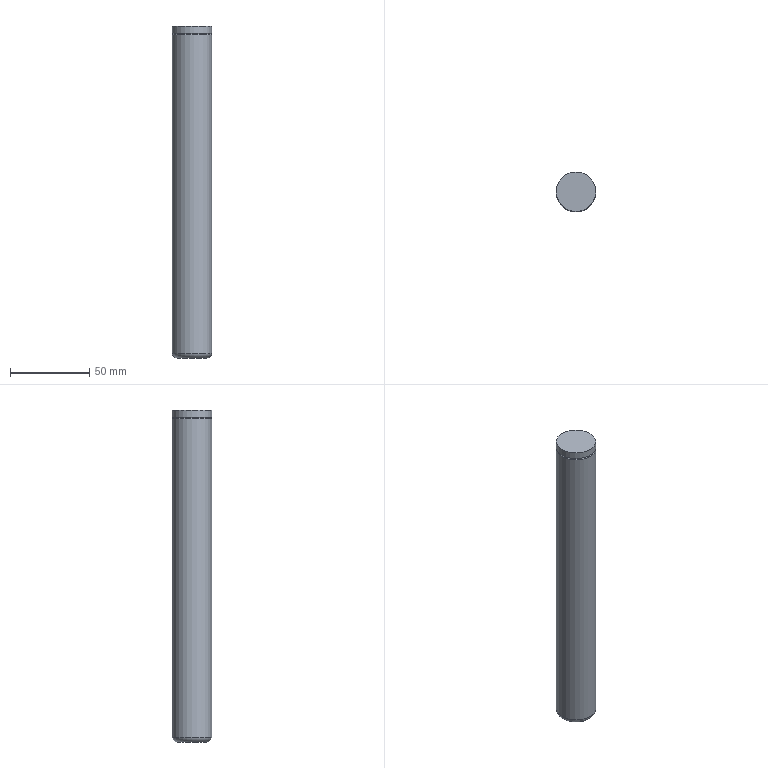Part | STEP file | 1 solid | 6 faces | box 25 x 25 x 210 mm | volume 102898 mm3 | plane 2 | cylinder 2 | torus 2 | commonest cylinder face diameters 25 x2
STEP:
#1=CARTESIAN_POINT('',(0.,0.,0.));
#2=DIRECTION('',(0.,0.,1.));
#3=DIRECTION('',(1.,0.,0.));
#4=AXIS2_PLACEMENT_3D('',#1,#2,#3);
#5=CARTESIAN_POINT('',(1301.872,580.48,-116.381));
#6=VERTEX_POINT('',#5);
#7=CARTESIAN_POINT('',(1311.247,580.48,-116.381));
#8=DIRECTION('',(0.,0.,-1.));
#9=DIRECTION('',(-1.,0.,0.));
#10=AXIS2_PLACEMENT_3D('',#7,#8,#9);
#11=CIRCLE('',#10,9.375);
#12=CARTESIAN_POINT('',(1311.247,580.48,-116.381));
#13=DIRECTION('',(0.,0.,-1.));
#14=DIRECTION('',(-1.,0.,0.));
#15=AXIS2_PLACEMENT_3D('',#12,#13,#14);
#16=PLANE('',#15);
#17=CARTESIAN_POINT('',(0.,0.));
#18=DIRECTION('',(1.,0.));
#19=AXIS2_PLACEMENT_2D('',#17,#18);
#20=CIRCLE('',#19,9.375);
#21=(GEOMETRIC_REPRESENTATION_CONTEXT(2)PARAMETRIC_REPRESENTATION_CONTEXT()REPRESENTATION_CONTEXT('',''));
#22=DEFINITIONAL_REPRESENTATION('',(#20),#21);
#23=PCURVE('',#16,#22);
#24=CARTESIAN_POINT('',(1311.247,580.48,-113.256));
#25=DIRECTION('',(0.,0.,-1.));
#26=DIRECTION('',(-1.,0.,0.));
#27=AXIS2_PLACEMENT_3D('',#24,#25,#26);
#28=TOROIDAL_SURFACE('',#27,9.375,3.125);
#29=CARTESIAN_POINT('',(0.,7.854));
#30=DIRECTION('',(1.,0.));
#31=VECTOR('',#30,1.);
#32=LINE('',#29,#31);
#33=(GEOMETRIC_REPRESENTATION_CONTEXT(2)PARAMETRIC_REPRESENTATION_CONTEXT()REPRESENTATION_CONTEXT('',''));
#34=DEFINITIONAL_REPRESENTATION('',(#32),#33);
#35=PCURVE('',#28,#34);
#36=SURFACE_CURVE('',#11,(#23,#35),.PCURVE_S1.);
#37=EDGE_CURVE('',#6,#6,#36,.T.);
#38=ORIENTED_EDGE('',*,*,#37,.T.);
#39=EDGE_LOOP('',(#38));
#40=FACE_BOUND('',#39,.T.);
#41=ADVANCED_FACE('',(#40),#16,.T.);
#42=CARTESIAN_POINT('',(1323.747,580.48,93.619));
#43=VERTEX_POINT('',#42);
#44=CARTESIAN_POINT('',(1311.247,580.48,93.619));
#45=DIRECTION('',(0.,0.,1.));
#46=DIRECTION('',(1.,0.,0.));
#47=AXIS2_PLACEMENT_3D('',#44,#45,#46);
#48=CIRCLE('',#47,12.5);
#49=CARTESIAN_POINT('',(1311.247,580.48,93.619));
#50=DIRECTION('',(0.,0.,1.));
#51=DIRECTION('',(1.,0.,0.));
#52=AXIS2_PLACEMENT_3D('',#49,#50,#51);
#53=PLANE('',#52);
#54=CARTESIAN_POINT('',(0.,0.));
#55=DIRECTION('',(1.,0.));
#56=AXIS2_PLACEMENT_2D('',#54,#55);
#57=CIRCLE('',#56,12.5);
#58=(GEOMETRIC_REPRESENTATION_CONTEXT(2)PARAMETRIC_REPRESENTATION_CONTEXT()REPRESENTATION_CONTEXT('',''));
#59=DEFINITIONAL_REPRESENTATION('',(#57),#58);
#60=PCURVE('',#53,#59);
#61=CARTESIAN_POINT('',(1311.247,580.48,-116.381));
#62=DIRECTION('',(0.,0.,1.));
#63=DIRECTION('',(1.,0.,0.));
#64=AXIS2_PLACEMENT_3D('',#61,#62,#63);
#65=CYLINDRICAL_SURFACE('',#64,12.5);
#66=CARTESIAN_POINT('',(0.,210.));
#67=DIRECTION('',(1.,0.));
#68=VECTOR('',#67,1.);
#69=LINE('',#66,#68);
#70=(GEOMETRIC_REPRESENTATION_CONTEXT(2)PARAMETRIC_REPRESENTATION_CONTEXT()REPRESENTATION_CONTEXT('',''));
#71=DEFINITIONAL_REPRESENTATION('',(#69),#70);
#72=PCURVE('',#65,#71);
#73=SURFACE_CURVE('',#48,(#60,#72),.PCURVE_S1.);
#74=EDGE_CURVE('',#43,#43,#73,.T.);
#75=ORIENTED_EDGE('',*,*,#74,.T.);
#76=EDGE_LOOP('',(#75));
#77=FACE_BOUND('',#76,.T.);
#78=ADVANCED_FACE('',(#77),#53,.T.);
#79=CARTESIAN_POINT('',(1323.747,580.48,89.119));
#80=VERTEX_POINT('',#79);
#81=CARTESIAN_POINT('',(1311.247,580.48,89.119));
#82=DIRECTION('',(0.,0.,1.));
#83=DIRECTION('',(1.,0.,0.));
#84=AXIS2_PLACEMENT_3D('',#81,#82,#83);
#85=CIRCLE('',#84,12.5);
#86=CARTESIAN_POINT('',(0.,205.5));
#87=DIRECTION('',(1.,0.));
#88=VECTOR('',#87,1.);
#89=LINE('',#86,#88);
#90=(GEOMETRIC_REPRESENTATION_CONTEXT(2)PARAMETRIC_REPRESENTATION_CONTEXT()REPRESENTATION_CONTEXT('',''));
#91=DEFINITIONAL_REPRESENTATION('',(#89),#90);
#92=PCURVE('',#65,#91);
#93=CARTESIAN_POINT('',(1311.247,580.48,88.619));
#94=DIRECTION('',(0.,0.,1.));
#95=DIRECTION('',(1.,0.,0.));
#96=AXIS2_PLACEMENT_3D('',#93,#94,#95);
#97=TOROIDAL_SURFACE('',#96,12.5,0.5);
#98=CARTESIAN_POINT('',(0.,1.571));
#99=DIRECTION('',(1.,0.));
#100=VECTOR('',#99,1.);
#101=LINE('',#98,#100);
#102=(GEOMETRIC_REPRESENTATION_CONTEXT(2)PARAMETRIC_REPRESENTATION_CONTEXT()REPRESENTATION_CONTEXT('',''));
#103=DEFINITIONAL_REPRESENTATION('',(#101),#102);
#104=PCURVE('',#97,#103);
#105=SURFACE_CURVE('',#85,(#92,#104),.PCURVE_S1.);
#106=EDGE_CURVE('',#80,#80,#105,.T.);
#107=ORIENTED_EDGE('',*,*,#106,.T.);
#108=CARTESIAN_POINT('',(1323.747,580.48,89.119));
#109=CARTESIAN_POINT('',(1323.747,580.48,93.619));
#110=B_SPLINE_CURVE_WITH_KNOTS('',1,(#108,#109),.UNSPECIFIED.,.F.,.F.,(2,2),(205.5,210.),.PIECEWISE_BEZIER_KNOTS.);
#111=CARTESIAN_POINT('',(6.283,0.));
#112=DIRECTION('',(0.,1.));
#113=VECTOR('',#112,1.);
#114=LINE('',#111,#113);
#115=(GEOMETRIC_REPRESENTATION_CONTEXT(2)PARAMETRIC_REPRESENTATION_CONTEXT()REPRESENTATION_CONTEXT('',''));
#116=DEFINITIONAL_REPRESENTATION('',(#114),#115);
#117=PCURVE('',#65,#116);
#118=CARTESIAN_POINT('',(0.,0.));
#119=DIRECTION('',(0.,1.));
#120=VECTOR('',#119,1.);
#121=LINE('',#118,#120);
#122=(GEOMETRIC_REPRESENTATION_CONTEXT(2)PARAMETRIC_REPRESENTATION_CONTEXT()REPRESENTATION_CONTEXT('',''));
#123=DEFINITIONAL_REPRESENTATION('',(#121),#122);
#124=PCURVE('',#65,#123);
#125=SEAM_CURVE('',#110,(#117,#124),.PCURVE_S1.);
#126=EDGE_CURVE('',#80,#43,#125,.T.);
#127=ORIENTED_EDGE('',*,*,#126,.T.);
#128=ORIENTED_EDGE('',*,*,#74,.F.);
#129=ORIENTED_EDGE('',*,*,#126,.F.);
#130=EDGE_LOOP('',(#107,#127,#128,#129));
#131=FACE_BOUND('',#130,.T.);
#132=ADVANCED_FACE('',(#131),#65,.T.);
#133=CARTESIAN_POINT('',(1323.747,580.48,88.119));
#134=VERTEX_POINT('',#133);
#135=CARTESIAN_POINT('',(1311.247,580.48,88.119));
#136=DIRECTION('',(0.,0.,1.));
#137=DIRECTION('',(1.,0.,0.));
#138=AXIS2_PLACEMENT_3D('',#135,#136,#137);
#139=CIRCLE('',#138,12.5);
#140=CARTESIAN_POINT('',(0.,4.712));
#141=DIRECTION('',(1.,0.));
#142=VECTOR('',#141,1.);
#143=LINE('',#140,#142);
#144=(GEOMETRIC_REPRESENTATION_CONTEXT(2)PARAMETRIC_REPRESENTATION_CONTEXT()REPRESENTATION_CONTEXT('',''));
#145=DEFINITIONAL_REPRESENTATION('',(#143),#144);
#146=PCURVE('',#97,#145);
#147=CARTESIAN_POINT('',(1311.247,580.48,-116.381));
#148=DIRECTION('',(0.,0.,1.));
#149=DIRECTION('',(1.,0.,0.));
#150=AXIS2_PLACEMENT_3D('',#147,#148,#149);
#151=CYLINDRICAL_SURFACE('',#150,12.5);
#152=CARTESIAN_POINT('',(0.,204.5));
#153=DIRECTION('',(1.,0.));
#154=VECTOR('',#153,1.);
#155=LINE('',#152,#154);
#156=(GEOMETRIC_REPRESENTATION_CONTEXT(2)PARAMETRIC_REPRESENTATION_CONTEXT()REPRESENTATION_CONTEXT('',''));
#157=DEFINITIONAL_REPRESENTATION('',(#155),#156);
#158=PCURVE('',#151,#157);
#159=SURFACE_CURVE('',#139,(#146,#158),.PCURVE_S1.);
#160=EDGE_CURVE('',#134,#134,#159,.T.);
#161=ORIENTED_EDGE('',*,*,#160,.F.);
#162=CARTESIAN_POINT('',(1323.747,580.48,89.119));
#163=CARTESIAN_POINT('',(1323.523,580.48,89.119));
#164=CARTESIAN_POINT('',(1323.299,580.48,89.002));
#165=CARTESIAN_POINT('',(1323.147,580.48,88.767));
#166=CARTESIAN_POINT('',(1323.147,580.48,88.471));
#167=CARTESIAN_POINT('',(1323.299,580.48,88.237));
#168=CARTESIAN_POINT('',(1323.523,580.48,88.119));
#169=CARTESIAN_POINT('',(1323.747,580.48,88.119));
#170=B_SPLINE_CURVE_WITH_KNOTS('',7,(#162,#163,#164,#165,#166,#167,#168,#169),.UNSPECIFIED.,.F.,.F.,(8,8),(1.571,4.712),.PIECEWISE_BEZIER_KNOTS.);
#171=CARTESIAN_POINT('',(0.,0.));
#172=DIRECTION('',(0.,1.));
#173=VECTOR('',#172,1.);
#174=LINE('',#171,#173);
#175=(GEOMETRIC_REPRESENTATION_CONTEXT(2)PARAMETRIC_REPRESENTATION_CONTEXT()REPRESENTATION_CONTEXT('',''));
#176=DEFINITIONAL_REPRESENTATION('',(#174),#175);
#177=PCURVE('',#97,#176);
#178=CARTESIAN_POINT('',(6.283,0.));
#179=DIRECTION('',(0.,1.));
#180=VECTOR('',#179,1.);
#181=LINE('',#178,#180);
#182=(GEOMETRIC_REPRESENTATION_CONTEXT(2)PARAMETRIC_REPRESENTATION_CONTEXT()REPRESENTATION_CONTEXT('',''));
#183=DEFINITIONAL_REPRESENTATION('',(#181),#182);
#184=PCURVE('',#97,#183);
#185=SEAM_CURVE('',#170,(#177,#184),.PCURVE_S1.);
#186=EDGE_CURVE('',#80,#134,#185,.T.);
#187=ORIENTED_EDGE('',*,*,#186,.F.);
#188=ORIENTED_EDGE('',*,*,#106,.T.);
#189=ORIENTED_EDGE('',*,*,#186,.T.);
#190=EDGE_LOOP('',(#161,#187,#188,#189));
#191=FACE_BOUND('',#190,.F.);
#192=ADVANCED_FACE('',(#191),#97,.F.);
#193=CARTESIAN_POINT('',(1298.747,580.48,-113.256));
#194=VERTEX_POINT('',#193);
#195=CARTESIAN_POINT('',(1323.747,580.48,-113.256));
#196=VERTEX_POINT('',#195);
#197=CARTESIAN_POINT('',(1311.247,580.48,-113.256));
#198=DIRECTION('',(0.,0.,1.));
#199=DIRECTION('',(-1.,0.,0.));
#200=AXIS2_PLACEMENT_3D('',#197,#198,#199);
#201=CIRCLE('',#200,12.5);
#202=CARTESIAN_POINT('',(3.142,3.125));
#203=DIRECTION('',(1.,0.));
#204=VECTOR('',#203,1.);
#205=LINE('',#202,#204);
#206=(GEOMETRIC_REPRESENTATION_CONTEXT(2)PARAMETRIC_REPRESENTATION_CONTEXT()REPRESENTATION_CONTEXT('',''));
#207=DEFINITIONAL_REPRESENTATION('',(#205),#206);
#208=PCURVE('',#151,#207);
#209=CARTESIAN_POINT('',(6.283,6.283));
#210=DIRECTION('',(-1.,0.));
#211=VECTOR('',#210,1.);
#212=LINE('',#209,#211);
#213=(GEOMETRIC_REPRESENTATION_CONTEXT(2)PARAMETRIC_REPRESENTATION_CONTEXT()REPRESENTATION_CONTEXT('',''));
#214=DEFINITIONAL_REPRESENTATION('',(#212),#213);
#215=PCURVE('',#28,#214);
#216=SURFACE_CURVE('',#201,(#208,#215),.PCURVE_S1.);
#217=EDGE_CURVE('',#194,#196,#216,.T.);
#218=ORIENTED_EDGE('',*,*,#217,.T.);
#219=CARTESIAN_POINT('',(1323.747,580.48,-113.256));
#220=CARTESIAN_POINT('',(1323.747,580.48,88.119));
#221=B_SPLINE_CURVE_WITH_KNOTS('',1,(#219,#220),.UNSPECIFIED.,.F.,.F.,(2,2),(3.125,204.5),.PIECEWISE_BEZIER_KNOTS.);
#222=CARTESIAN_POINT('',(6.283,0.));
#223=DIRECTION('',(0.,1.));
#224=VECTOR('',#223,1.);
#225=LINE('',#222,#224);
#226=(GEOMETRIC_REPRESENTATION_CONTEXT(2)PARAMETRIC_REPRESENTATION_CONTEXT()REPRESENTATION_CONTEXT('',''));
#227=DEFINITIONAL_REPRESENTATION('',(#225),#226);
#228=PCURVE('',#151,#227);
#229=CARTESIAN_POINT('',(0.,0.));
#230=DIRECTION('',(0.,1.));
#231=VECTOR('',#230,1.);
#232=LINE('',#229,#231);
#233=(GEOMETRIC_REPRESENTATION_CONTEXT(2)PARAMETRIC_REPRESENTATION_CONTEXT()REPRESENTATION_CONTEXT('',''));
#234=DEFINITIONAL_REPRESENTATION('',(#232),#233);
#235=PCURVE('',#151,#234);
#236=SEAM_CURVE('',#221,(#228,#235),.PCURVE_S1.);
#237=EDGE_CURVE('',#196,#134,#236,.T.);
#238=ORIENTED_EDGE('',*,*,#237,.T.);
#239=ORIENTED_EDGE('',*,*,#160,.F.);
#240=ORIENTED_EDGE('',*,*,#237,.F.);
#241=CARTESIAN_POINT('',(1311.247,580.48,-113.256));
#242=DIRECTION('',(0.,0.,1.));
#243=DIRECTION('',(-1.,0.,0.));
#244=AXIS2_PLACEMENT_3D('',#241,#242,#243);
#245=CIRCLE('',#244,12.5);
#246=CARTESIAN_POINT('',(-3.142,3.125));
#247=DIRECTION('',(1.,0.));
#248=VECTOR('',#247,1.);
#249=LINE('',#246,#248);
#250=(GEOMETRIC_REPRESENTATION_CONTEXT(2)PARAMETRIC_REPRESENTATION_CONTEXT()REPRESENTATION_CONTEXT('',''));
#251=DEFINITIONAL_REPRESENTATION('',(#249),#250);
#252=PCURVE('',#151,#251);
#253=CARTESIAN_POINT('',(6.283,6.283));
#254=DIRECTION('',(-1.,0.));
#255=VECTOR('',#254,1.);
#256=LINE('',#253,#255);
#257=(GEOMETRIC_REPRESENTATION_CONTEXT(2)PARAMETRIC_REPRESENTATION_CONTEXT()REPRESENTATION_CONTEXT('',''));
#258=DEFINITIONAL_REPRESENTATION('',(#256),#257);
#259=PCURVE('',#28,#258);
#260=SURFACE_CURVE('',#245,(#252,#259),.PCURVE_S1.);
#261=EDGE_CURVE('',#196,#194,#260,.T.);
#262=ORIENTED_EDGE('',*,*,#261,.T.);
#263=EDGE_LOOP('',(#218,#238,#239,#240,#262));
#264=FACE_BOUND('',#263,.T.);
#265=ADVANCED_FACE('',(#264),#151,.T.);
#266=ORIENTED_EDGE('',*,*,#37,.F.);
#267=CARTESIAN_POINT('',(1298.747,580.48,-113.256));
#268=CARTESIAN_POINT('',(1298.747,580.48,-114.091));
#269=CARTESIAN_POINT('',(1299.013,580.48,-114.905));
#270=CARTESIAN_POINT('',(1299.522,580.48,-115.606));
#271=CARTESIAN_POINT('',(1300.223,580.48,-116.115));
#272=CARTESIAN_POINT('',(1301.037,580.48,-116.381));
#273=CARTESIAN_POINT('',(1301.872,580.48,-116.381));
#274=(BOUNDED_CURVE()B_SPLINE_CURVE(6,(#267,#268,#269,#270,#271,#272,#273),.UNSPECIFIED.,.F.,.F.)B_SPLINE_CURVE_WITH_KNOTS((7,7),(0.,1.571),.PIECEWISE_BEZIER_KNOTS.)CURVE()GEOMETRIC_REPRESENTATION_ITEM()RATIONAL_B_SPLINE_CURVE((1.031,1.01,0.9979,0.994,0.9979,1.01,1.031))REPRESENTATION_ITEM(''));
#275=CARTESIAN_POINT('',(0.,6.283));
#276=DIRECTION('',(0.,1.));
#277=VECTOR('',#276,1.);
#278=LINE('',#275,#277);
#279=(GEOMETRIC_REPRESENTATION_CONTEXT(2)PARAMETRIC_REPRESENTATION_CONTEXT()REPRESENTATION_CONTEXT('',''));
#280=DEFINITIONAL_REPRESENTATION('',(#278),#279);
#281=PCURVE('',#28,#280);
#282=CARTESIAN_POINT('',(6.283,6.283));
#283=DIRECTION('',(0.,1.));
#284=VECTOR('',#283,1.);
#285=LINE('',#282,#284);
#286=(GEOMETRIC_REPRESENTATION_CONTEXT(2)PARAMETRIC_REPRESENTATION_CONTEXT()REPRESENTATION_CONTEXT('',''));
#287=DEFINITIONAL_REPRESENTATION('',(#285),#286);
#288=PCURVE('',#28,#287);
#289=SEAM_CURVE('',#274,(#281,#288),.PCURVE_S1.);
#290=EDGE_CURVE('',#194,#6,#289,.T.);
#291=ORIENTED_EDGE('',*,*,#290,.F.);
#292=ORIENTED_EDGE('',*,*,#261,.F.);
#293=ORIENTED_EDGE('',*,*,#217,.F.);
#294=ORIENTED_EDGE('',*,*,#290,.T.);
#295=EDGE_LOOP('',(#266,#291,#292,#293,#294));
#296=FACE_BOUND('',#295,.T.);
#297=ADVANCED_FACE('',(#296),#28,.T.);
#298=CLOSED_SHELL('',(#41,#78,#132,#192,#265,#297));
#299=MANIFOLD_SOLID_BREP('',#298);
#300=(LENGTH_UNIT()NAMED_UNIT(*)SI_UNIT(.MILLI.,.METRE.));
#301=UNCERTAINTY_MEASURE_WITH_UNIT(LENGTH_MEASURE(0.00001),#300,'','');
#302=(NAMED_UNIT(*)PLANE_ANGLE_UNIT()SI_UNIT($,.RADIAN.));
#303=(NAMED_UNIT(*)SI_UNIT($,.STERADIAN.)SOLID_ANGLE_UNIT());
#304=(GEOMETRIC_REPRESENTATION_CONTEXT(3)GLOBAL_UNCERTAINTY_ASSIGNED_CONTEXT((#301))GLOBAL_UNIT_ASSIGNED_CONTEXT((#300,#302,#303))REPRESENTATION_CONTEXT('',''));
#305=ADVANCED_BREP_SHAPE_REPRESENTATION('',(#4,#299),#304);